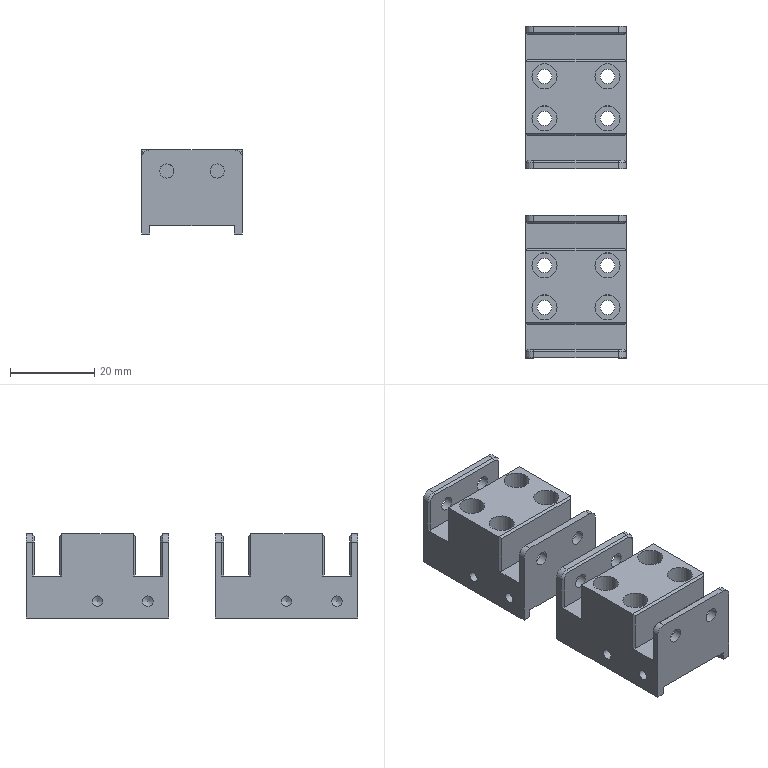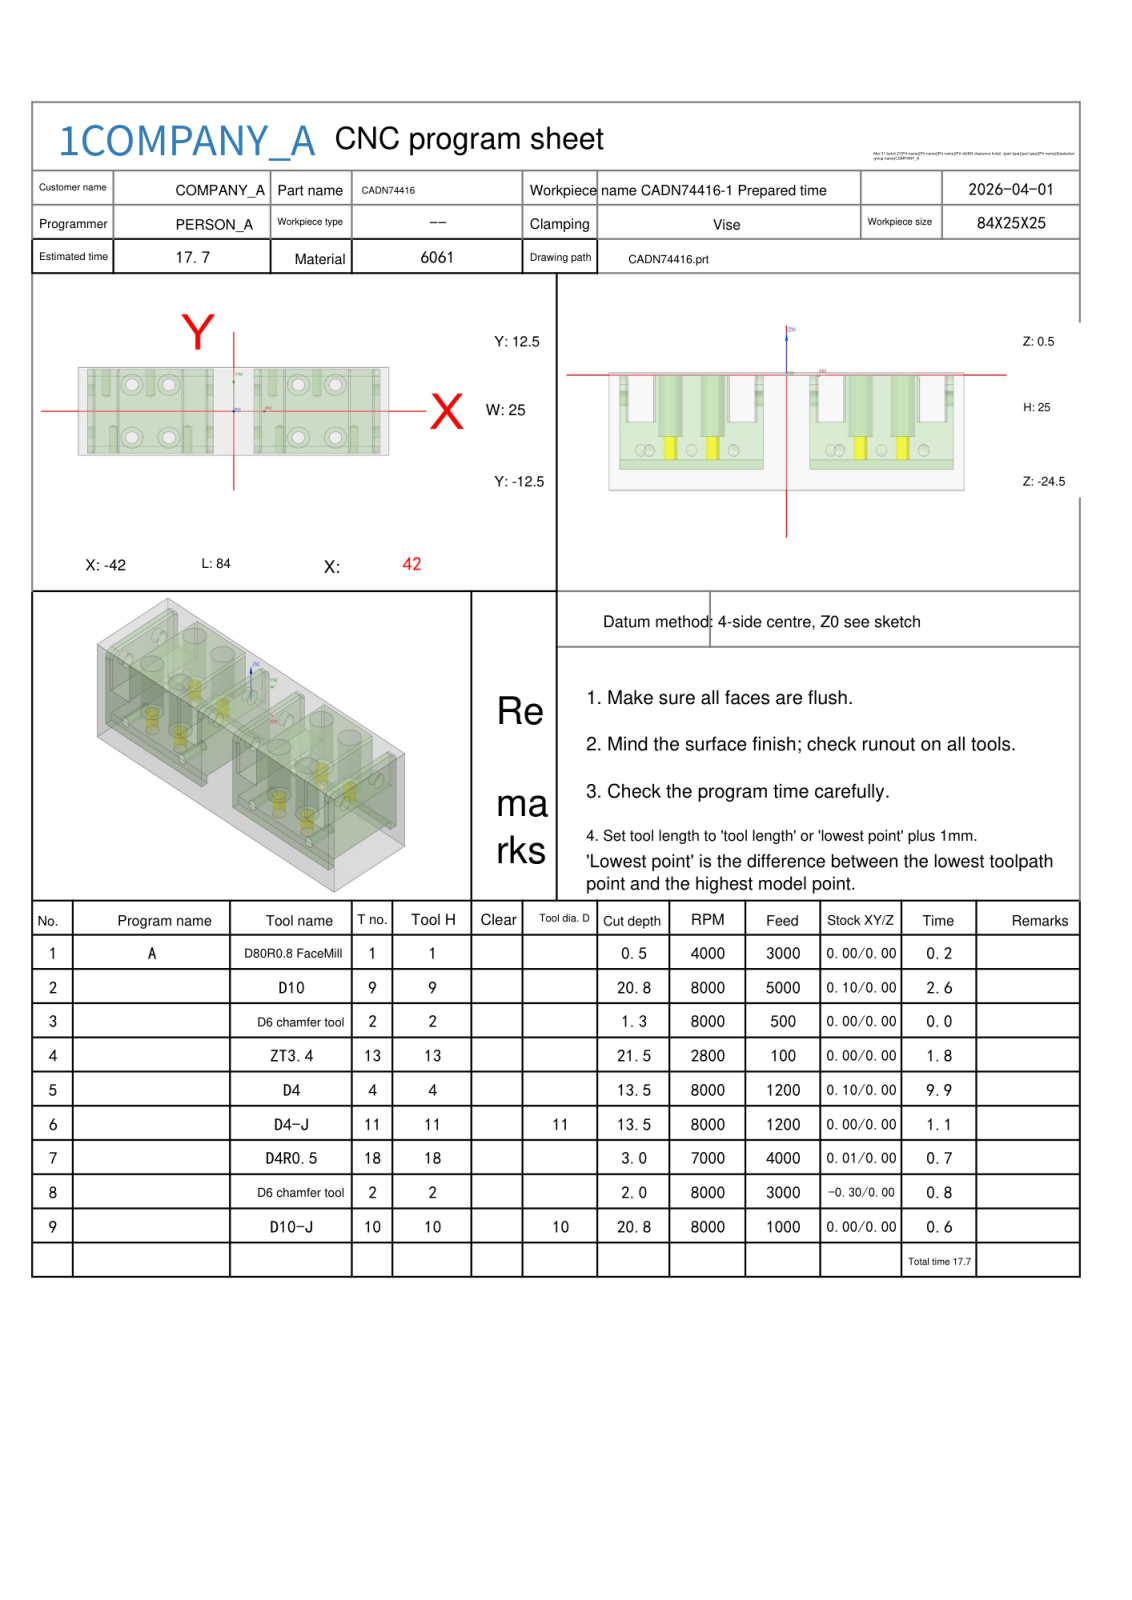NC program | NX | posted by the shop | part box 24 x 79 x 20 mm
Lines 795 to 4216 of 7697, first 2527 of 3422 lines:
N5 T04 M06
(D4  D=4. R=0. H=04 ce=0.10 di=0.10)
G00 G90 G54 X-10.5 Y17. M03 S6000
G43 H04 Z20.
M08
Z.253
G01 Z-.248 F1200.
Y12.4
X-11.43
X-11.4 Y12.37
Y-12.37
X-11.43 Y-12.4
X-9.57
X-9.6 Y-12.37
Y12.37
X-9.57 Y12.4
X-10.5
X-11.
Z.253
G00 Z.5
X-10.5 Y17.
Z.005
G01 Z-.495
Y12.4
X-11.43
X-11.4 Y12.37
Y-12.37
X-11.43 Y-12.4
X-9.57
X-9.6 Y-12.37
Y12.37
X-9.57 Y12.4
X-10.5
X-11.
Z.005
G00 Z.253
X-10.5 Y17.
Z-.243
G01 Z-.743
Y12.4
X-11.43
X-11.4 Y12.37
Y-12.37
X-11.43 Y-12.4
X-9.57
X-9.6 Y-12.37
Y12.37
X-9.57 Y12.4
X-10.5
X-11.
Z-.243
G00 Z.005
X-10.5 Y17.
Z-.49
G01 Z-.99
Y12.4
X-11.43
X-11.4 Y12.37
Y-12.37
X-11.43 Y-12.4
X-9.57
X-9.6 Y-12.37
Y12.37
X-9.57 Y12.4
X-10.5
X-11.
Z-.49
G00 Z-.243
X-10.5 Y17.
Z-.738
G01 Z-1.238
Y12.4
X-11.43
X-11.4 Y12.37
Y-12.37
X-11.43 Y-12.4
X-9.57
X-9.6 Y-12.37
Y12.37
X-9.57 Y12.4
X-10.5
X-11.
Z-.738
G00 Z-.49
X-10.5 Y17.
Z-.985
G01 Z-1.485
Y12.4
X-11.43
X-11.4 Y12.37
Y-12.37
X-11.43 Y-12.4
X-9.57
X-9.6 Y-12.37
Y12.37
X-9.57 Y12.4
X-10.5
X-11.
Z-.985
G00 Z-.738
X-10.5 Y17.
Z-1.233
G01 Z-1.733
Y12.4
X-11.43
X-11.4 Y12.37
Y-12.37
X-11.43 Y-12.4
X-9.57
X-9.6 Y-12.37
Y12.37
X-9.57 Y12.4
X-10.5
X-11.
Z-1.233
G00 Z-.985
X-10.5 Y17.
Z-1.48
G01 Z-1.98
Y12.4
X-11.43
X-11.4 Y12.37
Y-12.37
X-11.43 Y-12.4
X-9.57
X-9.6 Y-12.37
Y12.37
X-9.57 Y12.4
X-10.5
X-11.
Z-1.48
G00 Z-1.233
X-10.5 Y17.
Z-1.728
G01 Z-2.228
Y12.4
X-11.43
X-11.4 Y12.37
Y-12.37
X-11.43 Y-12.4
X-9.57
X-9.6 Y-12.37
Y12.37
X-9.57 Y12.4
X-10.5
X-11.
Z-1.728
G00 Z-1.48
X-10.5 Y17.
Z-1.975
G01 Z-2.475
Y12.4
X-11.43
X-11.4 Y12.37
Y-12.37
X-11.43 Y-12.4
X-9.57
X-9.6 Y-12.37
Y12.37
X-9.57 Y12.4
X-10.5
X-11.
Z-1.975
G00 Z-1.728
X-10.5 Y17.
Z-2.223
G01 Z-2.723
Y12.4
X-11.43
X-11.4 Y12.37
Y-12.37
X-11.43 Y-12.4
X-9.57
X-9.6 Y-12.37
Y12.37
X-9.57 Y12.4
X-10.5
X-11.
Z-2.223
G00 Z-1.975
X-10.5 Y17.
Z-2.47
G01 Z-2.97
Y12.4
X-11.43
X-11.4 Y12.37
Y-12.37
X-11.43 Y-12.4
X-9.57
X-9.6 Y-12.37
Y12.37
X-9.57 Y12.4
X-10.5
X-11.
Z-2.47
G00 Z-2.223
X-10.5 Y17.
Z-2.718
G01 Z-3.218
Y12.4
X-11.43
X-11.4 Y12.37
Y-12.37
X-11.43 Y-12.4
X-9.57
X-9.6 Y-12.37
Y12.37
X-9.57 Y12.4
X-10.5
X-11.
Z-2.718
G00 Z-2.47
X-10.5 Y17.
Z-2.965
G01 Z-3.465
Y12.4
X-11.43
X-11.4 Y12.37
Y-12.37
X-11.43 Y-12.4
X-9.57
X-9.6 Y-12.37
Y12.37
X-9.57 Y12.4
X-10.5
X-11.
Z-2.965
G00 Z-2.718
X-10.5 Y17.
Z-3.213
G01 Z-3.713
Y12.4
X-11.43
X-11.4 Y12.37
Y-12.37
X-11.43 Y-12.4
X-9.57
X-9.6 Y-12.37
Y12.37
X-9.57 Y12.4
X-10.5
X-11.
Z-3.213
G00 Z-2.965
X-10.5 Y17.
Z-3.46
G01 Z-3.96
Y12.4
X-11.43
X-11.4 Y12.37
Y-12.37
X-11.43 Y-12.4
X-9.57
X-9.6 Y-12.37
Y12.37
X-9.57 Y12.4
X-10.5
X-11.
Z-3.46
G00 Z-3.213
X-10.5 Y17.
Z-3.708
G01 Z-4.208
Y12.4
X-11.43
X-11.4 Y12.37
Y-12.37
X-11.43 Y-12.4
X-9.57
X-9.6 Y-12.37
Y12.37
X-9.57 Y12.4
X-10.5
X-11.
Z-3.708
G00 Z-3.46
X-10.5 Y17.
Z-3.955
G01 Z-4.455
Y12.4
X-11.43
X-11.4 Y12.37
Y-12.37
X-11.43 Y-12.4
X-9.57
X-9.6 Y-12.37
Y12.37
X-9.57 Y12.4
X-10.5
X-11.
Z-3.955
G00 Z-3.708
X-10.5 Y17.
Z-4.203
G01 Z-4.703
Y12.4
X-11.43
X-11.4 Y12.37
Y-12.37
X-11.43 Y-12.4
X-9.57
X-9.6 Y-12.37
Y12.37
X-9.57 Y12.4
X-10.5
X-11.
Z-4.203
G00 Z-3.955
X-10.5 Y17.
Z-4.45
G01 Z-4.95
Y12.4
X-11.43
X-11.4 Y12.37
Y-12.37
X-11.43 Y-12.4
X-9.57
X-9.6 Y-12.37
Y12.37
X-9.57 Y12.4
X-10.5
X-11.
Z-4.45
G00 Z-4.203
X-10.5 Y17.
Z-4.698
G01 Z-5.198
Y12.4
X-11.43
X-11.4 Y12.37
Y-12.37
X-11.43 Y-12.4
X-9.57
X-9.6 Y-12.37
Y12.37
X-9.57 Y12.4
X-10.5
X-11.
Z-4.698
G00 Z-4.45
X-10.5 Y17.
Z-4.945
G01 Z-5.445
Y12.4
X-11.43
X-11.4 Y12.37
Y-12.37
X-11.43 Y-12.4
X-9.57
X-9.6 Y-12.37
Y12.37
X-9.57 Y12.4
X-10.5
X-11.
Z-4.945
G00 Z-4.698
X-10.5 Y17.
Z-5.193
G01 Z-5.693
Y12.4
X-11.43
X-11.4 Y12.37
Y-12.37
X-11.43 Y-12.4
X-9.57
X-9.6 Y-12.37
Y12.37
X-9.57 Y12.4
X-10.5
X-11.
Z-5.193
G00 Z-4.945
X-10.5 Y17.
Z-5.44
G01 Z-5.94
Y12.4
X-11.43
X-11.4 Y12.37
Y-12.37
X-11.43 Y-12.4
X-9.57
X-9.6 Y-12.37
Y12.37
X-9.57 Y12.4
X-10.5
X-11.
Z-5.44
G00 Z-5.193
X-10.5 Y17.
Z-5.688
G01 Z-6.188
Y12.4
X-11.43
X-11.4 Y12.37
Y-12.37
X-11.43 Y-12.4
X-9.57
X-9.6 Y-12.37
Y12.37
X-9.57 Y12.4
X-10.5
X-11.
Z-5.688
G00 Z-5.44
X-10.5 Y17.
Z-5.935
G01 Z-6.435
Y12.4
X-11.43
X-11.4 Y12.37
Y-12.37
X-11.43 Y-12.4
X-9.57
X-9.6 Y-12.37
Y12.37
X-9.57 Y12.4
X-10.5
X-11.
Z-5.935
G00 Z-5.688
X-10.5 Y17.
Z-6.183
G01 Z-6.683
Y12.4
X-11.43
X-11.4 Y12.37
Y-12.37
X-11.43 Y-12.4
X-9.57
X-9.6 Y-12.37
Y12.37
X-9.57 Y12.4
X-10.5
X-11.
Z-6.183
G00 Z-5.935
X-10.5 Y17.
Z-6.43
G01 Z-6.93
Y12.4
X-11.43
X-11.4 Y12.37
Y-12.37
X-11.43 Y-12.4
X-9.57
X-9.6 Y-12.37
Y12.37
X-9.57 Y12.4
X-10.5
X-11.
Z-6.43
G00 Z-6.183
X-10.5 Y17.
Z-6.678
G01 Z-7.178
Y12.4
X-11.43
X-11.4 Y12.37
Y-12.37
X-11.43 Y-12.4
X-9.57
X-9.6 Y-12.37
Y12.37
X-9.57 Y12.4
X-10.5
X-11.
Z-6.678
G00 Z-6.43
X-10.5 Y17.
Z-6.925
G01 Z-7.425
Y12.4
X-11.43
X-11.4 Y12.37
Y-12.37
X-11.43 Y-12.4
X-9.57
X-9.6 Y-12.37
Y12.37
X-9.57 Y12.4
X-10.5
X-11.
Z-6.925
G00 Z-6.678
X-10.5 Y17.
Z-7.173
G01 Z-7.673
Y12.4
X-11.43
X-11.4 Y12.37
Y-12.37
X-11.43 Y-12.4
X-9.57
X-9.6 Y-12.37
Y12.37
X-9.57 Y12.4
X-10.5
X-11.
Z-7.173
G00 Z-6.925
X-10.5 Y17.
Z-7.42
G01 Z-7.92
Y12.4
X-11.43
X-11.4 Y12.37
Y-12.37
X-11.43 Y-12.4
X-9.57
X-9.6 Y-12.37
Y12.37
X-9.57 Y12.4
X-10.5
X-11.
Z-7.42
G00 Z-7.173
X-10.5 Y17.
Z-7.668
G01 Z-8.168
Y12.4
X-11.43
X-11.4 Y12.37
Y-12.37
X-11.43 Y-12.4
X-9.57
X-9.6 Y-12.37
Y12.37
X-9.57 Y12.4
X-10.5
X-11.
Z-7.668
G00 Z-7.42
X-10.5 Y17.
Z-7.915
G01 Z-8.415
Y12.4
X-11.43
X-11.4 Y12.37
Y-12.37
X-11.43 Y-12.4
X-9.57
X-9.6 Y-12.37
Y12.37
X-9.57 Y12.4
X-10.5
X-11.
Z-7.915
G00 Z-7.668
X-10.5 Y17.
Z-8.163
G01 Z-8.663
Y12.4
X-11.43
X-11.4 Y12.37
Y-12.37
X-11.43 Y-12.4
X-9.57
X-9.6 Y-12.37
Y12.37
X-9.57 Y12.4
X-10.5
X-11.
Z-8.163
G00 Z-7.915
X-10.5 Y17.
Z-8.41
G01 Z-8.91
Y12.4
X-11.43
X-11.4 Y12.37
Y-12.37
X-11.43 Y-12.4
X-9.57
X-9.6 Y-12.37
Y12.37
X-9.57 Y12.4
X-10.5
X-11.
Z-8.41
G00 Z-8.163
X-10.5 Y17.
Z-8.658
G01 Z-9.158
Y12.4
X-11.43
X-11.4 Y12.37
Y-12.37
X-11.43 Y-12.4
X-9.57
X-9.6 Y-12.37
Y12.37
X-9.57 Y12.4
X-10.5
X-11.
Z-8.658
G00 Z-8.41
X-10.5 Y17.
Z-8.905
G01 Z-9.405
Y12.4
X-11.43
X-11.4 Y12.37
Y-12.37
X-11.43 Y-12.4
X-9.57
X-9.6 Y-12.37
Y12.37
X-9.57 Y12.4
X-10.5
X-11.
Z-8.905
G00 Z-8.658
X-10.5 Y17.
Z-9.153
G01 Z-9.653
Y12.4
X-11.43
X-11.4 Y12.37
Y-12.37
X-11.43 Y-12.4
X-9.57
X-9.6 Y-12.37
Y12.37
X-9.57 Y12.4
X-10.5
X-11.
Z-9.153
G00 Z-8.905
X-10.5 Y17.
Z-9.4
G01 Z-9.9
Y12.4
X-11.43
X-11.4 Y12.37
Y-12.37
X-11.43 Y-12.4
X-9.57
X-9.6 Y-12.37
Y12.37
X-9.57 Y12.4
X-10.5
X-11.
Z-9.4
G00 Z20.
X34.5 Y17.
Z.253
G01 Z-.248
Y12.4
X33.57
X33.6 Y12.37
Y-12.37
X33.57 Y-12.4
X35.43
X35.4 Y-12.37
Y12.37
X35.43 Y12.4
X34.5
X34.
Z.253
G00 Z.5
X34.5 Y17.
Z.005
G01 Z-.495
Y12.4
X33.57
X33.6 Y12.37
Y-12.37
X33.57 Y-12.4
X35.43
X35.4 Y-12.37
Y12.37
X35.43 Y12.4
X34.5
X34.
Z.005
G00 Z.253
X34.5 Y17.
Z-.243
G01 Z-.743
Y12.4
X33.57
X33.6 Y12.37
Y-12.37
X33.57 Y-12.4
X35.43
X35.4 Y-12.37
Y12.37
X35.43 Y12.4
X34.5
X34.
Z-.243
G00 Z.005
X34.5 Y17.
Z-.49
G01 Z-.99
Y12.4
X33.57
X33.6 Y12.37
Y-12.37
X33.57 Y-12.4
X35.43
X35.4 Y-12.37
Y12.37
X35.43 Y12.4
X34.5
X34.
Z-.49
G00 Z-.243
X34.5 Y17.
Z-.738
G01 Z-1.238
Y12.4
X33.57
X33.6 Y12.37
Y-12.37
X33.57 Y-12.4
X35.43
X35.4 Y-12.37
Y12.37
X35.43 Y12.4
X34.5
X34.
Z-.738
G00 Z-.49
X34.5 Y17.
Z-.985
G01 Z-1.485
Y12.4
X33.57
X33.6 Y12.37
Y-12.37
X33.57 Y-12.4
X35.43
X35.4 Y-12.37
Y12.37
X35.43 Y12.4
X34.5
X34.
Z-.985
G00 Z-.738
X34.5 Y17.
Z-1.233
G01 Z-1.733
Y12.4
X33.57
X33.6 Y12.37
Y-12.37
X33.57 Y-12.4
X35.43
X35.4 Y-12.37
Y12.37
X35.43 Y12.4
X34.5
X34.
Z-1.233
G00 Z-.985
X34.5 Y17.
Z-1.48
G01 Z-1.98
Y12.4
X33.57
X33.6 Y12.37
Y-12.37
X33.57 Y-12.4
X35.43
X35.4 Y-12.37
Y12.37
X35.43 Y12.4
X34.5
X34.
Z-1.48
G00 Z-1.233
X34.5 Y17.
Z-1.728
G01 Z-2.228
Y12.4
X33.57
X33.6 Y12.37
Y-12.37
X33.57 Y-12.4
X35.43
X35.4 Y-12.37
Y12.37
X35.43 Y12.4
X34.5
X34.
Z-1.728
G00 Z-1.48
X34.5 Y17.
Z-1.975
G01 Z-2.475
Y12.4
X33.57
X33.6 Y12.37
Y-12.37
X33.57 Y-12.4
X35.43
X35.4 Y-12.37
Y12.37
X35.43 Y12.4
X34.5
X34.
Z-1.975
G00 Z-1.728
X34.5 Y17.
Z-2.223
G01 Z-2.723
Y12.4
X33.57
X33.6 Y12.37
Y-12.37
X33.57 Y-12.4
X35.43
X35.4 Y-12.37
Y12.37
X35.43 Y12.4
X34.5
X34.
Z-2.223
G00 Z-1.975
X34.5 Y17.
Z-2.47
G01 Z-2.97
Y12.4
X33.57
X33.6 Y12.37
Y-12.37
X33.57 Y-12.4
X35.43
X35.4 Y-12.37
Y12.37
X35.43 Y12.4
X34.5
X34.
Z-2.47
G00 Z-2.223
X34.5 Y17.
Z-2.718
G01 Z-3.218
Y12.4
X33.57
X33.6 Y12.37
Y-12.37
X33.57 Y-12.4
X35.43
X35.4 Y-12.37
Y12.37
X35.43 Y12.4
X34.5
X34.
Z-2.718
G00 Z-2.47
X34.5 Y17.
Z-2.965
G01 Z-3.465
Y12.4
X33.57
X33.6 Y12.37
Y-12.37
X33.57 Y-12.4
X35.43
X35.4 Y-12.37
Y12.37
X35.43 Y12.4
X34.5
X34.
Z-2.965
G00 Z-2.718
X34.5 Y17.
Z-3.213
G01 Z-3.713
Y12.4
X33.57
X33.6 Y12.37
Y-12.37
X33.57 Y-12.4
X35.43
X35.4 Y-12.37
Y12.37
X35.43 Y12.4
X34.5
X34.
Z-3.213
G00 Z-2.965
X34.5 Y17.
Z-3.46
G01 Z-3.96
Y12.4
X33.57
X33.6 Y12.37
Y-12.37
X33.57 Y-12.4
X35.43
X35.4 Y-12.37
Y12.37
X35.43 Y12.4
X34.5
X34.
Z-3.46
G00 Z-3.213
X34.5 Y17.
Z-3.708
G01 Z-4.208
Y12.4
X33.57
X33.6 Y12.37
Y-12.37
X33.57 Y-12.4
X35.43
X35.4 Y-12.37
Y12.37
X35.43 Y12.4
X34.5
X34.
Z-3.708
G00 Z-3.46
X34.5 Y17.
Z-3.955
G01 Z-4.455
Y12.4
X33.57
X33.6 Y12.37
Y-12.37
X33.57 Y-12.4
X35.43
X35.4 Y-12.37
Y12.37
X35.43 Y12.4
X34.5
X34.
Z-3.955
G00 Z-3.708
X34.5 Y17.
Z-4.203
G01 Z-4.703
Y12.4
X33.57
X33.6 Y12.37
Y-12.37
X33.57 Y-12.4
X35.43
X35.4 Y-12.37
Y12.37
X35.43 Y12.4
X34.5
X34.
Z-4.203
G00 Z-3.955
X34.5 Y17.
Z-4.45
G01 Z-4.95
Y12.4
X33.57
X33.6 Y12.37
Y-12.37
X33.57 Y-12.4
X35.43
X35.4 Y-12.37
Y12.37
X35.43 Y12.4
X34.5
X34.
Z-4.45
G00 Z-4.203
X34.5 Y17.
Z-4.698
G01 Z-5.198
Y12.4
X33.57
X33.6 Y12.37
Y-12.37
X33.57 Y-12.4
X35.43
X35.4 Y-12.37
Y12.37
X35.43 Y12.4
X34.5
X34.
Z-4.698
G00 Z-4.45
X34.5 Y17.
Z-4.945
G01 Z-5.445
Y12.4
X33.57
X33.6 Y12.37
Y-12.37
X33.57 Y-12.4
X35.43
X35.4 Y-12.37
Y12.37
X35.43 Y12.4
X34.5
X34.
Z-4.945
G00 Z-4.698
X34.5 Y17.
Z-5.193
G01 Z-5.693
Y12.4
X33.57
X33.6 Y12.37
Y-12.37
X33.57 Y-12.4
X35.43
X35.4 Y-12.37
Y12.37
X35.43 Y12.4
X34.5
X34.
Z-5.193
G00 Z-4.945
X34.5 Y17.
Z-5.44
G01 Z-5.94
Y12.4
X33.57
X33.6 Y12.37
Y-12.37
X33.57 Y-12.4
X35.43
X35.4 Y-12.37
Y12.37
X35.43 Y12.4
X34.5
X34.
Z-5.44
G00 Z-5.193
X34.5 Y17.
Z-5.688
G01 Z-6.188
Y12.4
X33.57
X33.6 Y12.37
Y-12.37
X33.57 Y-12.4
X35.43
X35.4 Y-12.37
Y12.37
X35.43 Y12.4
X34.5
X34.
Z-5.688
G00 Z-5.44
X34.5 Y17.
Z-5.935
G01 Z-6.435
Y12.4
X33.57
X33.6 Y12.37
Y-12.37
X33.57 Y-12.4
X35.43
X35.4 Y-12.37
Y12.37
X35.43 Y12.4
X34.5
X34.
Z-5.935
G00 Z-5.688
X34.5 Y17.
Z-6.183
G01 Z-6.683
Y12.4
X33.57
X33.6 Y12.37
Y-12.37
X33.57 Y-12.4
X35.43
X35.4 Y-12.37
Y12.37
X35.43 Y12.4
X34.5
X34.
Z-6.183
G00 Z-5.935
X34.5 Y17.
Z-6.43
G01 Z-6.93
Y12.4
X33.57
X33.6 Y12.37
Y-12.37
X33.57 Y-12.4
X35.43
X35.4 Y-12.37
Y12.37
X35.43 Y12.4
X34.5
X34.
Z-6.43
G00 Z-6.183
X34.5 Y17.
Z-6.678
G01 Z-7.178
Y12.4
X33.57
X33.6 Y12.37
Y-12.37
X33.57 Y-12.4
X35.43
X35.4 Y-12.37
Y12.37
X35.43 Y12.4
X34.5
X34.
Z-6.678
G00 Z-6.43
X34.5 Y17.
Z-6.925
G01 Z-7.425
Y12.4
X33.57
X33.6 Y12.37
Y-12.37
X33.57 Y-12.4
X35.43
X35.4 Y-12.37
Y12.37
X35.43 Y12.4
X34.5
X34.
Z-6.925
G00 Z-6.678
X34.5 Y17.
Z-7.173
G01 Z-7.673
Y12.4
X33.57
X33.6 Y12.37
Y-12.37
X33.57 Y-12.4
X35.43
X35.4 Y-12.37
Y12.37
X35.43 Y12.4
X34.5
X34.
Z-7.173
G00 Z-6.925
X34.5 Y17.
Z-7.42
G01 Z-7.92
Y12.4
X33.57
X33.6 Y12.37
Y-12.37
X33.57 Y-12.4
X35.43
X35.4 Y-12.37
Y12.37
X35.43 Y12.4
X34.5
X34.
Z-7.42
G00 Z-7.173
X34.5 Y17.
Z-7.668
G01 Z-8.168
Y12.4
X33.57
X33.6 Y12.37
Y-12.37
X33.57 Y-12.4
X35.43
X35.4 Y-12.37
Y12.37
X35.43 Y12.4
X34.5
X34.
Z-7.668
G00 Z-7.42
X34.5 Y17.
Z-7.915
G01 Z-8.415
Y12.4
X33.57
X33.6 Y12.37
Y-12.37
X33.57 Y-12.4
X35.43
X35.4 Y-12.37
Y12.37
X35.43 Y12.4
X34.5
X34.
Z-7.915
G00 Z-7.668
X34.5 Y17.
Z-8.163
G01 Z-8.663
Y12.4
X33.57
X33.6 Y12.37
Y-12.37
X33.57 Y-12.4
X35.43
X35.4 Y-12.37
Y12.37
X35.43 Y12.4
X34.5
X34.
Z-8.163
G00 Z-7.915
X34.5 Y17.
Z-8.41
G01 Z-8.91
Y12.4
X33.57
X33.6 Y12.37
Y-12.37
X33.57 Y-12.4
X35.43
X35.4 Y-12.37
Y12.37
X35.43 Y12.4
X34.5
X34.
Z-8.41
G00 Z-8.163
X34.5 Y17.
Z-8.658
G01 Z-9.158
Y12.4
X33.57
X33.6 Y12.37
Y-12.37
X33.57 Y-12.4
X35.43
X35.4 Y-12.37
Y12.37
X35.43 Y12.4
X34.5
X34.
Z-8.658
G00 Z-8.41
X34.5 Y17.
Z-8.905
G01 Z-9.405
Y12.4
X33.57
X33.6 Y12.37
Y-12.37
X33.57 Y-12.4
X35.43
X35.4 Y-12.37
Y12.37
X35.43 Y12.4
X34.5
X34.
Z-8.905
G00 Z-8.658
X34.5 Y17.
Z-9.153
G01 Z-9.653
Y12.4
X33.57
X33.6 Y12.37
Y-12.37
X33.57 Y-12.4
X35.43
X35.4 Y-12.37
Y12.37
X35.43 Y12.4
X34.5
X34.
Z-9.153
G00 Z-8.905
X34.5 Y17.
Z-9.4
G01 Z-9.9
Y12.4
X33.57
X33.6 Y12.37
Y-12.37
X33.57 Y-12.4
X35.43
X35.4 Y-12.37
Y12.37
X35.43 Y12.4
X34.5
X34.
Z-9.4
G00 Z20.
G00 G90 X-34.5 Y-17. M03 S6000
Z20.
Z.253
G01 Z-.248 F1200.
Y-12.4
X-33.57
X-33.6 Y-12.37
Y12.37
X-33.57 Y12.4
X-35.43
X-35.4 Y12.37
Y-12.37
X-35.43 Y-12.4
X-34.5
X-34.
Z.253
G00 Z.5
X-34.5 Y-17.
Z.005
G01 Z-.495
Y-12.4
X-33.57
X-33.6 Y-12.37
Y12.37
X-33.57 Y12.4
X-35.43
X-35.4 Y12.37
Y-12.37
X-35.43 Y-12.4
X-34.5
X-34.
Z.005
G00 Z.253
X-34.5 Y-17.
Z-.243
G01 Z-.743
Y-12.4
X-33.57
X-33.6 Y-12.37
Y12.37
X-33.57 Y12.4
X-35.43
X-35.4 Y12.37
Y-12.37
X-35.43 Y-12.4
X-34.5
X-34.
Z-.243
G00 Z.005
X-34.5 Y-17.
Z-.49
G01 Z-.99
Y-12.4
X-33.57
X-33.6 Y-12.37
Y12.37
X-33.57 Y12.4
X-35.43
X-35.4 Y12.37
Y-12.37
X-35.43 Y-12.4
X-34.5
X-34.
Z-.49
G00 Z-.243
X-34.5 Y-17.
Z-.738
G01 Z-1.238
Y-12.4
X-33.57
X-33.6 Y-12.37
Y12.37
X-33.57 Y12.4
X-35.43
X-35.4 Y12.37
Y-12.37
X-35.43 Y-12.4
X-34.5
X-34.
Z-.738
G00 Z-.49
X-34.5 Y-17.
Z-.985
G01 Z-1.485
Y-12.4
X-33.57
X-33.6 Y-12.37
Y12.37
X-33.57 Y12.4
X-35.43
X-35.4 Y12.37
Y-12.37
X-35.43 Y-12.4
X-34.5
X-34.
Z-.985
G00 Z-.738
X-34.5 Y-17.
Z-1.233
G01 Z-1.733
Y-12.4
X-33.57
X-33.6 Y-12.37
Y12.37
X-33.57 Y12.4
X-35.43
X-35.4 Y12.37
Y-12.37
X-35.43 Y-12.4
X-34.5
X-34.
Z-1.233
G00 Z-.985
X-34.5 Y-17.
Z-1.48
G01 Z-1.98
Y-12.4
X-33.57
X-33.6 Y-12.37
Y12.37
X-33.57 Y12.4
X-35.43
X-35.4 Y12.37
Y-12.37
X-35.43 Y-12.4
X-34.5
X-34.
Z-1.48
G00 Z-1.233
X-34.5 Y-17.
Z-1.728
G01 Z-2.228
Y-12.4
X-33.57
X-33.6 Y-12.37
Y12.37
X-33.57 Y12.4
X-35.43
X-35.4 Y12.37
Y-12.37
X-35.43 Y-12.4
X-34.5
X-34.
Z-1.728
G00 Z-1.48
X-34.5 Y-17.
Z-1.975
G01 Z-2.475
Y-12.4
X-33.57
X-33.6 Y-12.37
Y12.37
X-33.57 Y12.4
X-35.43
X-35.4 Y12.37
Y-12.37
X-35.43 Y-12.4
X-34.5
X-34.
Z-1.975
G00 Z-1.728
X-34.5 Y-17.
Z-2.223
G01 Z-2.723
Y-12.4
X-33.57
X-33.6 Y-12.37
Y12.37
X-33.57 Y12.4
X-35.43
X-35.4 Y12.37
Y-12.37
X-35.43 Y-12.4
X-34.5
X-34.
Z-2.223
G00 Z-1.975
X-34.5 Y-17.
Z-2.47
G01 Z-2.97
Y-12.4
X-33.57
X-33.6 Y-12.37
Y12.37
X-33.57 Y12.4
X-35.43
X-35.4 Y12.37
Y-12.37
X-35.43 Y-12.4
X-34.5
X-34.
Z-2.47
G00 Z-2.223
X-34.5 Y-17.
Z-2.718
G01 Z-3.218
Y-12.4
X-33.57
X-33.6 Y-12.37
Y12.37
X-33.57 Y12.4
X-35.43
X-35.4 Y12.37
Y-12.37
X-35.43 Y-12.4
X-34.5
X-34.
Z-2.718
G00 Z-2.47
X-34.5 Y-17.
Z-2.965
G01 Z-3.465
Y-12.4
X-33.57
X-33.6 Y-12.37
Y12.37
X-33.57 Y12.4
X-35.43
X-35.4 Y12.37
Y-12.37
X-35.43 Y-12.4
X-34.5
X-34.
Z-2.965
G00 Z-2.718
X-34.5 Y-17.
Z-3.213
G01 Z-3.713
Y-12.4
X-33.57
X-33.6 Y-12.37
Y12.37
X-33.57 Y12.4
X-35.43
X-35.4 Y12.37
Y-12.37
X-35.43 Y-12.4
X-34.5
X-34.
Z-3.213
G00 Z-2.965
X-34.5 Y-17.
Z-3.46
G01 Z-3.96
Y-12.4
X-33.57
X-33.6 Y-12.37
Y12.37
X-33.57 Y12.4
X-35.43
X-35.4 Y12.37
Y-12.37
X-35.43 Y-12.4
X-34.5
X-34.
Z-3.46
G00 Z-3.213
X-34.5 Y-17.
Z-3.708
G01 Z-4.208
Y-12.4
X-33.57
X-33.6 Y-12.37
Y12.37
X-33.57 Y12.4
X-35.43
X-35.4 Y12.37
Y-12.37
X-35.43 Y-12.4
X-34.5
X-34.
Z-3.708
G00 Z-3.46
X-34.5 Y-17.
Z-3.955
G01 Z-4.455
Y-12.4
X-33.57
X-33.6 Y-12.37
Y12.37
X-33.57 Y12.4
X-35.43
X-35.4 Y12.37
Y-12.37
X-35.43 Y-12.4
X-34.5
X-34.
Z-3.955
G00 Z-3.708
X-34.5 Y-17.
Z-4.203
G01 Z-4.703
Y-12.4
X-33.57
X-33.6 Y-12.37
Y12.37
X-33.57 Y12.4
X-35.43
X-35.4 Y12.37
Y-12.37
X-35.43 Y-12.4
X-34.5
X-34.
Z-4.203
G00 Z-3.955
X-34.5 Y-17.
Z-4.45
G01 Z-4.95
Y-12.4
X-33.57
X-33.6 Y-12.37
Y12.37
X-33.57 Y12.4
X-35.43
X-35.4 Y12.37
Y-12.37
X-35.43 Y-12.4
X-34.5
X-34.
Z-4.45
G00 Z-4.203
X-34.5 Y-17.
Z-4.698
G01 Z-5.198
Y-12.4
X-33.57
X-33.6 Y-12.37
Y12.37
X-33.57 Y12.4
X-35.43
X-35.4 Y12.37
Y-12.37
X-35.43 Y-12.4
X-34.5
X-34.
Z-4.698
G00 Z-4.45
X-34.5 Y-17.
Z-4.945
G01 Z-5.445
Y-12.4
X-33.57
X-33.6 Y-12.37
Y12.37
X-33.57 Y12.4
X-35.43
X-35.4 Y12.37
Y-12.37
X-35.43 Y-12.4
X-34.5
X-34.
Z-4.945
G00 Z-4.698
X-34.5 Y-17.
Z-5.193
G01 Z-5.693
Y-12.4
X-33.57
X-33.6 Y-12.37
Y12.37
X-33.57 Y12.4
X-35.43
X-35.4 Y12.37
Y-12.37
X-35.43 Y-12.4
X-34.5
X-34.
Z-5.193
G00 Z-4.945
X-34.5 Y-17.
Z-5.44
G01 Z-5.94
Y-12.4
X-33.57
X-33.6 Y-12.37
Y12.37
X-33.57 Y12.4
X-35.43
X-35.4 Y12.37
Y-12.37
X-35.43 Y-12.4
X-34.5
X-34.
Z-5.44
G00 Z-5.193
X-34.5 Y-17.
Z-5.688
G01 Z-6.188
Y-12.4
X-33.57
X-33.6 Y-12.37
Y12.37
X-33.57 Y12.4
X-35.43
X-35.4 Y12.37
Y-12.37
X-35.43 Y-12.4
X-34.5
X-34.
Z-5.688
G00 Z-5.44
X-34.5 Y-17.
Z-5.935
G01 Z-6.435
Y-12.4
X-33.57
X-33.6 Y-12.37
Y12.37
X-33.57 Y12.4
X-35.43
X-35.4 Y12.37
Y-12.37
X-35.43 Y-12.4
X-34.5
X-34.
Z-5.935
G00 Z-5.688
X-34.5 Y-17.
Z-6.183
G01 Z-6.683
Y-12.4
X-33.57
X-33.6 Y-12.37
Y12.37
X-33.57 Y12.4
X-35.43
X-35.4 Y12.37
Y-12.37
X-35.43 Y-12.4
X-34.5
X-34.
Z-6.183
G00 Z-5.935
X-34.5 Y-17.
Z-6.43
G01 Z-6.93
Y-12.4
X-33.57
X-33.6 Y-12.37
Y12.37
X-33.57 Y12.4
X-35.43
X-35.4 Y12.37
Y-12.37
X-35.43 Y-12.4
X-34.5
X-34.
Z-6.43
G00 Z-6.183
X-34.5 Y-17.
Z-6.678
G01 Z-7.178
Y-12.4
X-33.57
X-33.6 Y-12.37
Y12.37
X-33.57 Y12.4
X-35.43
X-35.4 Y12.37
Y-12.37
X-35.43 Y-12.4
X-34.5
X-34.
Z-6.678
G00 Z-6.43
X-34.5 Y-17.
Z-6.925
G01 Z-7.425
Y-12.4
X-33.57
X-33.6 Y-12.37
Y12.37
X-33.57 Y12.4
X-35.43
X-35.4 Y12.37
Y-12.37
X-35.43 Y-12.4
X-34.5
X-34.
Z-6.925
G00 Z-6.678
X-34.5 Y-17.
Z-7.173
G01 Z-7.673
Y-12.4
X-33.57
X-33.6 Y-12.37
Y12.37
X-33.57 Y12.4
X-35.43
X-35.4 Y12.37
Y-12.37
X-35.43 Y-12.4
X-34.5
X-34.
Z-7.173
G00 Z-6.925
X-34.5 Y-17.
Z-7.42
G01 Z-7.92
Y-12.4
X-33.57
X-33.6 Y-12.37
Y12.37
X-33.57 Y12.4
X-35.43
X-35.4 Y12.37
Y-12.37
X-35.43 Y-12.4
X-34.5
X-34.
Z-7.42
G00 Z-7.173
X-34.5 Y-17.
Z-7.668
G01 Z-8.168
Y-12.4
X-33.57
X-33.6 Y-12.37
Y12.37
X-33.57 Y12.4
X-35.43
X-35.4 Y12.37
Y-12.37
X-35.43 Y-12.4
X-34.5
X-34.
Z-7.668
G00 Z-7.42
X-34.5 Y-17.
Z-7.915
G01 Z-8.415
Y-12.4
X-33.57
X-33.6 Y-12.37
Y12.37
X-33.57 Y12.4
X-35.43
X-35.4 Y12.37
Y-12.37
X-35.43 Y-12.4
X-34.5
X-34.
Z-7.915
G00 Z-7.668
X-34.5 Y-17.
Z-8.163
G01 Z-8.663
Y-12.4
X-33.57
X-33.6 Y-12.37
Y12.37
X-33.57 Y12.4
X-35.43
X-35.4 Y12.37
Y-12.37
X-35.43 Y-12.4
X-34.5
X-34.
Z-8.163
G00 Z-7.915
X-34.5 Y-17.
Z-8.41
G01 Z-8.91
Y-12.4
X-33.57
X-33.6 Y-12.37
Y12.37
X-33.57 Y12.4
X-35.43
X-35.4 Y12.37
Y-12.37
X-35.43 Y-12.4
X-34.5
X-34.
Z-8.41
G00 Z-8.163
X-34.5 Y-17.
Z-8.658
G01 Z-9.158
Y-12.4
X-33.57
X-33.6 Y-12.37
Y12.37
X-33.57 Y12.4
X-35.43
X-35.4 Y12.37
Y-12.37
X-35.43 Y-12.4
X-34.5
X-34.
Z-8.658
G00 Z-8.41
X-34.5 Y-17.
Z-8.905
G01 Z-9.405
Y-12.4
X-33.57
X-33.6 Y-12.37
Y12.37
X-33.57 Y12.4
X-35.43
X-35.4 Y12.37
Y-12.37
X-35.43 Y-12.4
X-34.5
X-34.
Z-8.905
G00 Z-8.658
X-34.5 Y-17.
Z-9.153
G01 Z-9.653
Y-12.4
X-33.57
X-33.6 Y-12.37
Y12.37
X-33.57 Y12.4
X-35.43
X-35.4 Y12.37
Y-12.37
X-35.43 Y-12.4
X-34.5
X-34.
Z-9.153
G00 Z-8.905
X-34.5 Y-17.
Z-9.4
G01 Z-9.9
Y-12.4
X-33.57
X-33.6 Y-12.37
Y12.37
X-33.57 Y12.4
X-35.43
X-35.4 Y12.37
Y-12.37
X-35.43 Y-12.4
X-34.5
X-34.
Z-9.4
G00 Z20.
X10.5 Y-17.
Z.253
G01 Z-.248
Y-12.4
X11.43
X11.4 Y-12.37
Y12.37
X11.43 Y12.4
X9.57
X9.6 Y12.37
Y-12.37
X9.57 Y-12.4
X10.5
X11.
Z.253
G00 Z.5
X10.5 Y-17.
Z.005
G01 Z-.495
Y-12.4
X11.43
X11.4 Y-12.37
Y12.37
X11.43 Y12.4
X9.57
X9.6 Y12.37
Y-12.37
X9.57 Y-12.4
X10.5
X11.
Z.005
G00 Z.253
X10.5 Y-17.
Z-.243
G01 Z-.743
Y-12.4
X11.43
X11.4 Y-12.37
Y12.37
X11.43 Y12.4
X9.57
X9.6 Y12.37
Y-12.37
X9.57 Y-12.4
X10.5
X11.
Z-.243
G00 Z.005
X10.5 Y-17.
Z-.49
G01 Z-.99
Y-12.4
X11.43
X11.4 Y-12.37
Y12.37
X11.43 Y12.4
X9.57
X9.6 Y12.37
Y-12.37
X9.57 Y-12.4
X10.5
X11.
Z-.49
G00 Z-.243
X10.5 Y-17.
Z-.738
G01 Z-1.238
Y-12.4
X11.43
X11.4 Y-12.37
Y12.37
X11.43 Y12.4
X9.57
X9.6 Y12.37
Y-12.37
X9.57 Y-12.4
X10.5
X11.
Z-.738
G00 Z-.49
X10.5 Y-17.
Z-.985
G01 Z-1.485
Y-12.4
X11.43
X11.4 Y-12.37
Y12.37
X11.43 Y12.4
X9.57
X9.6 Y12.37
Y-12.37
X9.57 Y-12.4
X10.5
X11.
Z-.985
G00 Z-.738
X10.5 Y-17.
Z-1.233
G01 Z-1.733
Y-12.4
X11.43
X11.4 Y-12.37
Y12.37
X11.43 Y12.4
X9.57
X9.6 Y12.37
Y-12.37
X9.57 Y-12.4
X10.5
X11.
Z-1.233
G00 Z-.985
X10.5 Y-17.
Z-1.48
G01 Z-1.98
Y-12.4
X11.43
X11.4 Y-12.37
Y12.37
X11.43 Y12.4
X9.57
X9.6 Y12.37
Y-12.37
X9.57 Y-12.4
X10.5
X11.
Z-1.48
G00 Z-1.233
X10.5 Y-17.
Z-1.728
G01 Z-2.228
Y-12.4
X11.43
X11.4 Y-12.37
Y12.37
X11.43 Y12.4
X9.57
X9.6 Y12.37
Y-12.37
X9.57 Y-12.4
X10.5
X11.
Z-1.728
G00 Z-1.48
X10.5 Y-17.
Z-1.975
G01 Z-2.475
Y-12.4
X11.43
X11.4 Y-12.37
Y12.37
X11.43 Y12.4
X9.57
X9.6 Y12.37
Y-12.37
X9.57 Y-12.4
X10.5
X11.
Z-1.975
G00 Z-1.728
X10.5 Y-17.
Z-2.223
G01 Z-2.723
Y-12.4
X11.43
X11.4 Y-12.37
Y12.37
X11.43 Y12.4
X9.57
X9.6 Y12.37
Y-12.37
X9.57 Y-12.4
X10.5
X11.
Z-2.223
G00 Z-1.975
X10.5 Y-17.
Z-2.47
G01 Z-2.97
Y-12.4
X11.43
X11.4 Y-12.37
Y12.37
X11.43 Y12.4
X9.57
X9.6 Y12.37
Y-12.37
X9.57 Y-12.4
X10.5
X11.
Z-2.47
G00 Z-2.223
X10.5 Y-17.
Z-2.718
G01 Z-3.218
Y-12.4
X11.43
X11.4 Y-12.37
Y12.37
X11.43 Y12.4
X9.57
X9.6 Y12.37
Y-12.37
X9.57 Y-12.4
X10.5
X11.
Z-2.718
G00 Z-2.47
X10.5 Y-17.
Z-2.965
G01 Z-3.465
Y-12.4
X11.43
X11.4 Y-12.37
Y12.37
X11.43 Y12.4
X9.57
X9.6 Y12.37
Y-12.37
X9.57 Y-12.4
X10.5
X11.
Z-2.965
G00 Z-2.718
X10.5 Y-17.
Z-3.213
G01 Z-3.713
Y-12.4
X11.43
X11.4 Y-12.37
Y12.37
X11.43 Y12.4
X9.57
X9.6 Y12.37
Y-12.37
X9.57 Y-12.4
X10.5
X11.
Z-3.213
G00 Z-2.965
X10.5 Y-17.
Z-3.46
G01 Z-3.96
Y-12.4
X11.43
X11.4 Y-12.37
Y12.37
X11.43 Y12.4
X9.57
X9.6 Y12.37
Y-12.37
X9.57 Y-12.4
X10.5
X11.
Z-3.46
G00 Z-3.213
X10.5 Y-17.
Z-3.708
G01 Z-4.208
Y-12.4
X11.43
X11.4 Y-12.37
Y12.37
X11.43 Y12.4
X9.57
X9.6 Y12.37
Y-12.37
X9.57 Y-12.4
X10.5
X11.
Z-3.708
G00 Z-3.46
X10.5 Y-17.
Z-3.955
G01 Z-4.455
Y-12.4
X11.43
X11.4 Y-12.37
Y12.37
X11.43 Y12.4
X9.57
X9.6 Y12.37
Y-12.37
X9.57 Y-12.4
X10.5
X11.
Z-3.955
G00 Z-3.708
X10.5 Y-17.
Z-4.203
G01 Z-4.703
Y-12.4
X11.43
X11.4 Y-12.37
Y12.37
X11.43 Y12.4
X9.57
X9.6 Y12.37
Y-12.37
X9.57 Y-12.4
X10.5
X11.
Z-4.203
G00 Z-3.955
X10.5 Y-17.
Z-4.45
G01 Z-4.95
Y-12.4
X11.43
X11.4 Y-12.37
Y12.37
X11.43 Y12.4
X9.57
X9.6 Y12.37
Y-12.37
X9.57 Y-12.4
X10.5
X11.
Z-4.45
G00 Z-4.203
X10.5 Y-17.
Z-4.698
G01 Z-5.198
Y-12.4
X11.43
X11.4 Y-12.37
Y12.37
X11.43 Y12.4
X9.57
X9.6 Y12.37
Y-12.37
X9.57 Y-12.4
X10.5
X11.
Z-4.698
G00 Z-4.45
X10.5 Y-17.
Z-4.945
G01 Z-5.445
Y-12.4
X11.43
X11.4 Y-12.37
Y12.37
X11.43 Y12.4
X9.57
X9.6 Y12.37
Y-12.37
X9.57 Y-12.4
X10.5
X11.
Z-4.945
G00 Z-4.698
X10.5 Y-17.
Z-5.193
G01 Z-5.693
Y-12.4
X11.43
X11.4 Y-12.37
Y12.37
X11.43 Y12.4
X9.57
X9.6 Y12.37
Y-12.37
X9.57 Y-12.4
X10.5
X11.
Z-5.193
G00 Z-4.945
X10.5 Y-17.
Z-5.44
G01 Z-5.94
Y-12.4
X11.43
X11.4 Y-12.37
Y12.37
X11.43 Y12.4
X9.57
X9.6 Y12.37
Y-12.37
X9.57 Y-12.4
X10.5
X11.
Z-5.44
G00 Z-5.193
X10.5 Y-17.
Z-5.688
G01 Z-6.188
Y-12.4
X11.43
X11.4 Y-12.37
Y12.37
X11.43 Y12.4
X9.57
X9.6 Y12.37
Y-12.37
X9.57 Y-12.4
X10.5
X11.
Z-5.688
G00 Z-5.44
X10.5 Y-17.
Z-5.935
G01 Z-6.435
Y-12.4
X11.43
X11.4 Y-12.37
Y12.37
X11.43 Y12.4
X9.57
X9.6 Y12.37
Y-12.37
X9.57 Y-12.4
X10.5
X11.
Z-5.935
G00 Z-5.688
X10.5 Y-17.
Z-6.183
G01 Z-6.683
Y-12.4
X11.43
X11.4 Y-12.37
Y12.37
X11.43 Y12.4
X9.57
X9.6 Y12.37
Y-12.37
X9.57 Y-12.4
X10.5
X11.
Z-6.183
G00 Z-5.935
X10.5 Y-17.
Z-6.43
G01 Z-6.93
Y-12.4
X11.43
X11.4 Y-12.37
Y12.37
X11.43 Y12.4
X9.57
X9.6 Y12.37
Y-12.37
X9.57 Y-12.4
X10.5
X11.
Z-6.43
G00 Z-6.183
X10.5 Y-17.
Z-6.678
G01 Z-7.178
Y-12.4
X11.43
X11.4 Y-12.37
Y12.37
X11.43 Y12.4
X9.57
X9.6 Y12.37
Y-12.37
X9.57 Y-12.4
X10.5
X11.
Z-6.678
G00 Z-6.43
X10.5 Y-17.
Z-6.925
G01 Z-7.425
Y-12.4
X11.43
X11.4 Y-12.37
Y12.37
X11.43 Y12.4
X9.57
X9.6 Y12.37
Y-12.37
X9.57 Y-12.4
X10.5
X11.
Z-6.925
G00 Z-6.678
X10.5 Y-17.
Z-7.173
G01 Z-7.673
Y-12.4
X11.43
X11.4 Y-12.37
Y12.37
X11.43 Y12.4
X9.57
X9.6 Y12.37
Y-12.37
X9.57 Y-12.4
X10.5
X11.
Z-7.173
G00 Z-6.925
X10.5 Y-17.
Z-7.42
G01 Z-7.92
Y-12.4
X11.43
X11.4 Y-12.37
Y12.37
X11.43 Y12.4
X9.57
X9.6 Y12.37
Y-12.37
X9.57 Y-12.4
X10.5
X11.
Z-7.42
G00 Z-7.173
X10.5 Y-17.
Z-7.668
G01 Z-8.168
Y-12.4
X11.43
X11.4 Y-12.37
Y12.37
X11.43 Y12.4
X9.57
X9.6 Y12.37
Y-12.37
X9.57 Y-12.4
X10.5
X11.
Z-7.668
G00 Z-7.42
X10.5 Y-17.
Z-7.915
G01 Z-8.415
Y-12.4
X11.43
X11.4 Y-12.37
Y12.37
X11.43 Y12.4
X9.57
X9.6 Y12.37
Y-12.37
X9.57 Y-12.4
X10.5
X11.
Z-7.915
G00 Z-7.668
X10.5 Y-17.
Z-8.163
G01 Z-8.663
Y-12.4
X11.43
X11.4 Y-12.37
Y12.37
X11.43 Y12.4
X9.57
X9.6 Y12.37
Y-12.37
X9.57 Y-12.4
X10.5
X11.
Z-8.163
G00 Z-7.915
X10.5 Y-17.
Z-8.41
G01 Z-8.91
Y-12.4
X11.43
X11.4 Y-12.37
Y12.37
X11.43 Y12.4
X9.57
X9.6 Y12.37
Y-12.37
X9.57 Y-12.4
X10.5
X11.
Z-8.41
G00 Z-8.163
X10.5 Y-17.
Z-8.658
G01 Z-9.158
Y-12.4
X11.43
X11.4 Y-12.37
Y12.37
X11.43 Y12.4
X9.57
X9.6 Y12.37
Y-12.37
X9.57 Y-12.4
X10.5
X11.
Z-8.658
G00 Z-8.41
X10.5 Y-17.
Z-8.905
G01 Z-9.405
Y-12.4
X11.43
X11.4 Y-12.37
Y12.37
X11.43 Y12.4
X9.57
X9.6 Y12.37